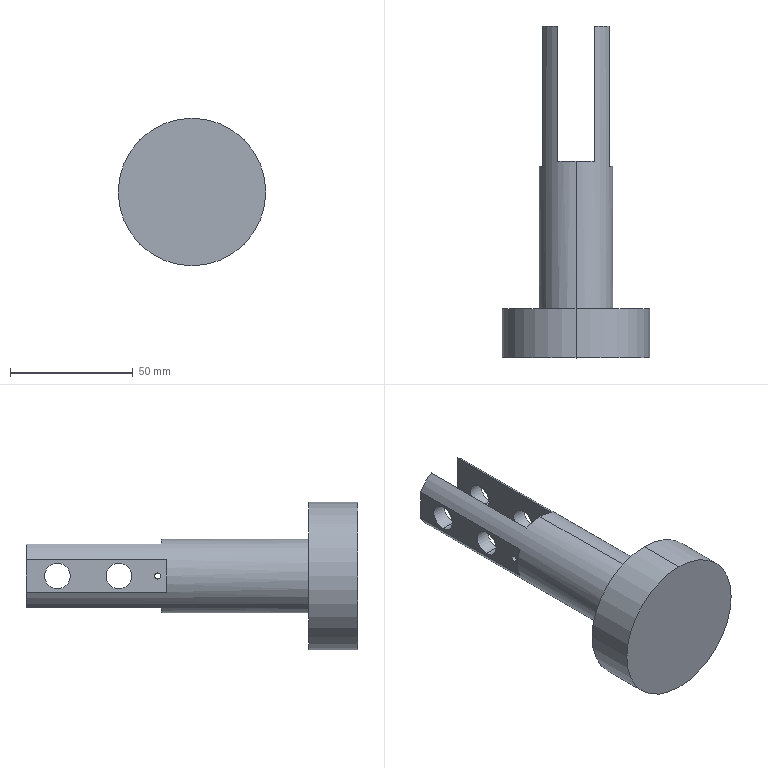Part | SolidWorks | features ICE 3, HoleWzd 2, Extrusion 1 | 1 solid | 27 faces | box 60 x 135 x 60 mm | volume 110518 mm3 | cylinder 16 | plane 11 | commonest cylinder face diameters 10.5 x8 2.5 x4 30 x2 60 x2
STEP:
#1=CARTESIAN_POINT('',(13.5,81.4,-1.25));
#2=VERTEX_POINT('',#1);
#3=CARTESIAN_POINT('',(13.5,81.4,1.25));
#4=VERTEX_POINT('',#3);
#5=CARTESIAN_POINT('',(13.5,81.4,0.));
#6=DIRECTION('',(-1.,0.,0.));
#7=DIRECTION('',(0.,0.,1.));
#8=AXIS2_PLACEMENT_3D('',#5,#6,#7);
#9=CIRCLE('',#8,1.25);
#10=EDGE_CURVE('',#2,#4,#9,.T.);
#11=ORIENTED_EDGE('',*,*,#10,.F.);
#12=CARTESIAN_POINT('',(7.5,81.4,-1.25));
#13=VERTEX_POINT('',#12);
#14=CARTESIAN_POINT('',(-13.5,81.4,-1.25));
#15=DIRECTION('',(-1.,0.,0.));
#16=VECTOR('',#15,1000.);
#17=LINE('',#14,#16);
#18=EDGE_CURVE('',#2,#13,#17,.T.);
#19=ORIENTED_EDGE('',*,*,#18,.T.);
#20=CARTESIAN_POINT('',(7.5,81.4,1.25));
#21=VERTEX_POINT('',#20);
#22=CARTESIAN_POINT('',(7.5,81.4,0.));
#23=DIRECTION('',(1.,0.,0.));
#24=DIRECTION('',(0.,0.,-1.));
#25=AXIS2_PLACEMENT_3D('',#22,#23,#24);
#26=CIRCLE('',#25,1.25);
#27=EDGE_CURVE('',#21,#13,#26,.T.);
#28=ORIENTED_EDGE('',*,*,#27,.F.);
#29=CARTESIAN_POINT('',(-13.5,81.4,1.25));
#30=DIRECTION('',(-1.,0.,0.));
#31=VECTOR('',#30,1000.);
#32=LINE('',#29,#31);
#33=EDGE_CURVE('',#4,#21,#32,.T.);
#34=ORIENTED_EDGE('',*,*,#33,.F.);
#35=EDGE_LOOP('',(#11,#19,#28,#34));
#36=FACE_OUTER_BOUND('',#35,.T.);
#37=CARTESIAN_POINT('',(-13.5,81.4,0.));
#38=DIRECTION('',(-1.,0.,0.));
#39=DIRECTION('',(0.,0.,1.));
#40=AXIS2_PLACEMENT_3D('',#37,#38,#39);
#41=CYLINDRICAL_SURFACE('',#40,1.25);
#42=ADVANCED_FACE('',(#36),#41,.F.);
#43=CARTESIAN_POINT('',(-7.5,81.4,-1.25));
#44=VERTEX_POINT('',#43);
#45=CARTESIAN_POINT('',(-7.5,81.4,1.25));
#46=VERTEX_POINT('',#45);
#47=CARTESIAN_POINT('',(-7.5,81.4,0.));
#48=DIRECTION('',(-1.,0.,0.));
#49=DIRECTION('',(0.,0.,1.));
#50=AXIS2_PLACEMENT_3D('',#47,#48,#49);
#51=CIRCLE('',#50,1.25);
#52=EDGE_CURVE('',#44,#46,#51,.T.);
#53=ORIENTED_EDGE('',*,*,#52,.F.);
#54=CARTESIAN_POINT('',(-13.5,81.4,-1.25));
#55=VERTEX_POINT('',#54);
#56=CARTESIAN_POINT('',(-13.5,81.4,-1.25));
#57=DIRECTION('',(-1.,0.,0.));
#58=VECTOR('',#57,1000.);
#59=LINE('',#56,#58);
#60=EDGE_CURVE('',#44,#55,#59,.T.);
#61=ORIENTED_EDGE('',*,*,#60,.T.);
#62=CARTESIAN_POINT('',(-13.5,81.4,1.25));
#63=VERTEX_POINT('',#62);
#64=CARTESIAN_POINT('',(-13.5,81.4,0.));
#65=DIRECTION('',(-1.,0.,0.));
#66=DIRECTION('',(0.,0.,1.));
#67=AXIS2_PLACEMENT_3D('',#64,#65,#66);
#68=CIRCLE('',#67,1.25);
#69=EDGE_CURVE('',#55,#63,#68,.T.);
#70=ORIENTED_EDGE('',*,*,#69,.T.);
#71=CARTESIAN_POINT('',(-13.5,81.4,1.25));
#72=DIRECTION('',(-1.,0.,0.));
#73=VECTOR('',#72,1000.);
#74=LINE('',#71,#73);
#75=EDGE_CURVE('',#46,#63,#74,.T.);
#76=ORIENTED_EDGE('',*,*,#75,.F.);
#77=EDGE_LOOP('',(#53,#61,#70,#76));
#78=FACE_OUTER_BOUND('',#77,.T.);
#79=CARTESIAN_POINT('',(-13.5,81.4,0.));
#80=DIRECTION('',(-1.,0.,0.));
#81=DIRECTION('',(0.,0.,1.));
#82=AXIS2_PLACEMENT_3D('',#79,#80,#81);
#83=CYLINDRICAL_SURFACE('',#82,1.25);
#84=ADVANCED_FACE('',(#78),#83,.F.);
#85=CARTESIAN_POINT('',(-13.5,97.25,5.25));
#86=VERTEX_POINT('',#85);
#87=CARTESIAN_POINT('',(-13.5,97.25,-5.25));
#88=VERTEX_POINT('',#87);
#89=CARTESIAN_POINT('',(-13.5,97.25,0.));
#90=DIRECTION('',(1.,0.,0.));
#91=DIRECTION('',(0.,1.,0.));
#92=AXIS2_PLACEMENT_3D('',#89,#90,#91);
#93=CIRCLE('',#92,5.25);
#94=EDGE_CURVE('',#86,#88,#93,.T.);
#95=ORIENTED_EDGE('',*,*,#94,.F.);
#96=CARTESIAN_POINT('',(-7.5,97.25,5.25));
#97=VERTEX_POINT('',#96);
#98=CARTESIAN_POINT('',(13.5,97.25,5.25));
#99=DIRECTION('',(1.,0.,0.));
#100=VECTOR('',#99,1000.);
#101=LINE('',#98,#100);
#102=EDGE_CURVE('',#86,#97,#101,.T.);
#103=ORIENTED_EDGE('',*,*,#102,.T.);
#104=CARTESIAN_POINT('',(-7.5,97.25,-5.25));
#105=VERTEX_POINT('',#104);
#106=CARTESIAN_POINT('',(-7.5,97.25,0.));
#107=DIRECTION('',(-1.,0.,0.));
#108=DIRECTION('',(0.,0.,1.));
#109=AXIS2_PLACEMENT_3D('',#106,#107,#108);
#110=CIRCLE('',#109,5.25);
#111=EDGE_CURVE('',#105,#97,#110,.T.);
#112=ORIENTED_EDGE('',*,*,#111,.F.);
#113=CARTESIAN_POINT('',(13.5,97.25,-5.25));
#114=DIRECTION('',(1.,0.,0.));
#115=VECTOR('',#114,1000.);
#116=LINE('',#113,#115);
#117=EDGE_CURVE('',#88,#105,#116,.T.);
#118=ORIENTED_EDGE('',*,*,#117,.F.);
#119=EDGE_LOOP('',(#95,#103,#112,#118));
#120=FACE_OUTER_BOUND('',#119,.T.);
#121=CARTESIAN_POINT('',(13.5,97.25,0.));
#122=DIRECTION('',(1.,0.,0.));
#123=DIRECTION('',(0.,0.,-1.));
#124=AXIS2_PLACEMENT_3D('',#121,#122,#123);
#125=CYLINDRICAL_SURFACE('',#124,5.25);
#126=ADVANCED_FACE('',(#120),#125,.F.);
#127=CARTESIAN_POINT('',(7.5,97.25,5.25));
#128=VERTEX_POINT('',#127);
#129=CARTESIAN_POINT('',(7.5,97.25,-5.25));
#130=VERTEX_POINT('',#129);
#131=CARTESIAN_POINT('',(7.5,97.25,0.));
#132=DIRECTION('',(1.,0.,0.));
#133=DIRECTION('',(0.,0.,-1.));
#134=AXIS2_PLACEMENT_3D('',#131,#132,#133);
#135=CIRCLE('',#134,5.25);
#136=EDGE_CURVE('',#128,#130,#135,.T.);
#137=ORIENTED_EDGE('',*,*,#136,.F.);
#138=CARTESIAN_POINT('',(13.5,97.25,5.25));
#139=VERTEX_POINT('',#138);
#140=CARTESIAN_POINT('',(13.5,97.25,5.25));
#141=DIRECTION('',(1.,0.,0.));
#142=VECTOR('',#141,1000.);
#143=LINE('',#140,#142);
#144=EDGE_CURVE('',#128,#139,#143,.T.);
#145=ORIENTED_EDGE('',*,*,#144,.T.);
#146=CARTESIAN_POINT('',(13.5,97.25,-5.25));
#147=VERTEX_POINT('',#146);
#148=CARTESIAN_POINT('',(13.5,97.25,0.));
#149=DIRECTION('',(1.,0.,0.));
#150=DIRECTION('',(0.,0.,-1.));
#151=AXIS2_PLACEMENT_3D('',#148,#149,#150);
#152=CIRCLE('',#151,5.25);
#153=EDGE_CURVE('',#139,#147,#152,.T.);
#154=ORIENTED_EDGE('',*,*,#153,.T.);
#155=CARTESIAN_POINT('',(13.5,97.25,-5.25));
#156=DIRECTION('',(1.,0.,0.));
#157=VECTOR('',#156,1000.);
#158=LINE('',#155,#157);
#159=EDGE_CURVE('',#130,#147,#158,.T.);
#160=ORIENTED_EDGE('',*,*,#159,.F.);
#161=EDGE_LOOP('',(#137,#145,#154,#160));
#162=FACE_OUTER_BOUND('',#161,.T.);
#163=CARTESIAN_POINT('',(13.5,97.25,0.));
#164=DIRECTION('',(1.,0.,0.));
#165=DIRECTION('',(0.,0.,-1.));
#166=AXIS2_PLACEMENT_3D('',#163,#164,#165);
#167=CYLINDRICAL_SURFACE('',#166,5.25);
#168=ADVANCED_FACE('',(#162),#167,.F.);
#169=CARTESIAN_POINT('',(7.5,122.25,5.25));
#170=VERTEX_POINT('',#169);
#171=CARTESIAN_POINT('',(7.5,122.25,-5.25));
#172=VERTEX_POINT('',#171);
#173=CARTESIAN_POINT('',(7.5,122.25,0.));
#174=DIRECTION('',(1.,0.,0.));
#175=DIRECTION('',(0.,0.,-1.));
#176=AXIS2_PLACEMENT_3D('',#173,#174,#175);
#177=CIRCLE('',#176,5.25);
#178=EDGE_CURVE('',#170,#172,#177,.T.);
#179=ORIENTED_EDGE('',*,*,#178,.F.);
#180=CARTESIAN_POINT('',(13.5,122.25,5.25));
#181=VERTEX_POINT('',#180);
#182=CARTESIAN_POINT('',(13.5,122.25,5.25));
#183=DIRECTION('',(1.,0.,0.));
#184=VECTOR('',#183,1000.);
#185=LINE('',#182,#184);
#186=EDGE_CURVE('',#170,#181,#185,.T.);
#187=ORIENTED_EDGE('',*,*,#186,.T.);
#188=CARTESIAN_POINT('',(13.5,122.25,-5.25));
#189=VERTEX_POINT('',#188);
#190=CARTESIAN_POINT('',(13.5,122.25,0.));
#191=DIRECTION('',(1.,0.,0.));
#192=DIRECTION('',(0.,0.,-1.));
#193=AXIS2_PLACEMENT_3D('',#190,#191,#192);
#194=CIRCLE('',#193,5.25);
#195=EDGE_CURVE('',#181,#189,#194,.T.);
#196=ORIENTED_EDGE('',*,*,#195,.T.);
#197=CARTESIAN_POINT('',(13.5,122.25,-5.25));
#198=DIRECTION('',(1.,0.,0.));
#199=VECTOR('',#198,1000.);
#200=LINE('',#197,#199);
#201=EDGE_CURVE('',#172,#189,#200,.T.);
#202=ORIENTED_EDGE('',*,*,#201,.F.);
#203=EDGE_LOOP('',(#179,#187,#196,#202));
#204=FACE_OUTER_BOUND('',#203,.T.);
#205=CARTESIAN_POINT('',(13.5,122.25,0.));
#206=DIRECTION('',(1.,0.,0.));
#207=DIRECTION('',(0.,0.,-1.));
#208=AXIS2_PLACEMENT_3D('',#205,#206,#207);
#209=CYLINDRICAL_SURFACE('',#208,5.25);
#210=ADVANCED_FACE('',(#204),#209,.F.);
#211=CARTESIAN_POINT('',(-13.5,122.25,5.25));
#212=VERTEX_POINT('',#211);
#213=CARTESIAN_POINT('',(-13.5,122.25,-5.25));
#214=VERTEX_POINT('',#213);
#215=CARTESIAN_POINT('',(-13.5,122.25,0.));
#216=DIRECTION('',(1.,0.,0.));
#217=DIRECTION('',(0.,1.,0.));
#218=AXIS2_PLACEMENT_3D('',#215,#216,#217);
#219=CIRCLE('',#218,5.25);
#220=EDGE_CURVE('',#212,#214,#219,.T.);
#221=ORIENTED_EDGE('',*,*,#220,.F.);
#222=CARTESIAN_POINT('',(-7.5,122.25,5.25));
#223=VERTEX_POINT('',#222);
#224=CARTESIAN_POINT('',(13.5,122.25,5.25));
#225=DIRECTION('',(1.,0.,0.));
#226=VECTOR('',#225,1000.);
#227=LINE('',#224,#226);
#228=EDGE_CURVE('',#212,#223,#227,.T.);
#229=ORIENTED_EDGE('',*,*,#228,.T.);
#230=CARTESIAN_POINT('',(-7.5,122.25,-5.25));
#231=VERTEX_POINT('',#230);
#232=CARTESIAN_POINT('',(-7.5,122.25,0.));
#233=DIRECTION('',(-1.,0.,0.));
#234=DIRECTION('',(0.,0.,1.));
#235=AXIS2_PLACEMENT_3D('',#232,#233,#234);
#236=CIRCLE('',#235,5.25);
#237=EDGE_CURVE('',#231,#223,#236,.T.);
#238=ORIENTED_EDGE('',*,*,#237,.F.);
#239=CARTESIAN_POINT('',(13.5,122.25,-5.25));
#240=DIRECTION('',(1.,0.,0.));
#241=VECTOR('',#240,1000.);
#242=LINE('',#239,#241);
#243=EDGE_CURVE('',#214,#231,#242,.T.);
#244=ORIENTED_EDGE('',*,*,#243,.F.);
#245=EDGE_LOOP('',(#221,#229,#238,#244));
#246=FACE_OUTER_BOUND('',#245,.T.);
#247=CARTESIAN_POINT('',(13.5,122.25,0.));
#248=DIRECTION('',(1.,0.,0.));
#249=DIRECTION('',(0.,0.,-1.));
#250=AXIS2_PLACEMENT_3D('',#247,#248,#249);
#251=CYLINDRICAL_SURFACE('',#250,5.25);
#252=ADVANCED_FACE('',(#246),#251,.F.);
#253=CARTESIAN_POINT('',(7.5,80.,12.99));
#254=VERTEX_POINT('',#253);
#255=CARTESIAN_POINT('',(0.,80.,15.));
#256=VERTEX_POINT('',#255);
#257=CARTESIAN_POINT('',(0.,80.,0.));
#258=DIRECTION('',(0.,-1.,0.));
#259=DIRECTION('',(0.,0.,-1.));
#260=AXIS2_PLACEMENT_3D('',#257,#258,#259);
#261=CIRCLE('',#260,15.);
#262=EDGE_CURVE('',#254,#256,#261,.T.);
#263=ORIENTED_EDGE('',*,*,#262,.T.);
#264=CARTESIAN_POINT('',(0.,20.,15.));
#265=VERTEX_POINT('',#264);
#266=CARTESIAN_POINT('',(0.,135.,15.));
#267=DIRECTION('',(0.,-1.,0.));
#268=VECTOR('',#267,1000.);
#269=LINE('',#266,#268);
#270=EDGE_CURVE('',#256,#265,#269,.T.);
#271=ORIENTED_EDGE('',*,*,#270,.T.);
#272=CARTESIAN_POINT('',(0.,20.,-15.));
#273=VERTEX_POINT('',#272);
#274=CARTESIAN_POINT('',(0.,20.,0.));
#275=DIRECTION('',(0.,1.,0.));
#276=DIRECTION('',(0.,0.,1.));
#277=AXIS2_PLACEMENT_3D('',#274,#275,#276);
#278=CIRCLE('',#277,15.);
#279=EDGE_CURVE('',#265,#273,#278,.T.);
#280=ORIENTED_EDGE('',*,*,#279,.T.);
#281=CARTESIAN_POINT('',(0.,80.,-15.));
#282=VERTEX_POINT('',#281);
#283=CARTESIAN_POINT('',(0.,135.,-15.));
#284=DIRECTION('',(0.,-1.,0.));
#285=VECTOR('',#284,1000.);
#286=LINE('',#283,#285);
#287=EDGE_CURVE('',#282,#273,#286,.T.);
#288=ORIENTED_EDGE('',*,*,#287,.F.);
#289=CARTESIAN_POINT('',(7.5,80.,-12.99));
#290=VERTEX_POINT('',#289);
#291=CARTESIAN_POINT('',(0.,80.,0.));
#292=DIRECTION('',(0.,-1.,0.));
#293=DIRECTION('',(0.,0.,-1.));
#294=AXIS2_PLACEMENT_3D('',#291,#292,#293);
#295=CIRCLE('',#294,15.);
#296=EDGE_CURVE('',#282,#290,#295,.T.);
#297=ORIENTED_EDGE('',*,*,#296,.T.);
#298=CARTESIAN_POINT('',(7.5,135.,-12.99));
#299=VERTEX_POINT('',#298);
#300=CARTESIAN_POINT('',(7.5,135.,-12.99));
#301=DIRECTION('',(0.,1.,0.));
#302=VECTOR('',#301,1000.);
#303=LINE('',#300,#302);
#304=EDGE_CURVE('',#290,#299,#303,.T.);
#305=ORIENTED_EDGE('',*,*,#304,.T.);
#306=CARTESIAN_POINT('',(13.5,135.,-6.538));
#307=VERTEX_POINT('',#306);
#308=CARTESIAN_POINT('',(0.,135.,0.));
#309=DIRECTION('',(0.,1.,0.));
#310=DIRECTION('',(0.,0.,1.));
#311=AXIS2_PLACEMENT_3D('',#308,#309,#310);
#312=CIRCLE('',#311,15.);
#313=EDGE_CURVE('',#307,#299,#312,.T.);
#314=ORIENTED_EDGE('',*,*,#313,.F.);
#315=CARTESIAN_POINT('',(13.5,78.,-6.538));
#316=VERTEX_POINT('',#315);
#317=CARTESIAN_POINT('',(13.5,135.,-6.538));
#318=DIRECTION('',(0.,-1.,0.));
#319=VECTOR('',#318,1000.);
#320=LINE('',#317,#319);
#321=EDGE_CURVE('',#307,#316,#320,.T.);
#322=ORIENTED_EDGE('',*,*,#321,.T.);
#323=CARTESIAN_POINT('',(13.5,78.,6.538));
#324=VERTEX_POINT('',#323);
#325=CARTESIAN_POINT('',(0.,78.,0.));
#326=DIRECTION('',(0.,-1.,0.));
#327=DIRECTION('',(0.,0.,-1.));
#328=AXIS2_PLACEMENT_3D('',#325,#326,#327);
#329=CIRCLE('',#328,15.);
#330=EDGE_CURVE('',#316,#324,#329,.T.);
#331=ORIENTED_EDGE('',*,*,#330,.T.);
#332=CARTESIAN_POINT('',(13.5,135.,6.538));
#333=VERTEX_POINT('',#332);
#334=CARTESIAN_POINT('',(13.5,135.,6.538));
#335=DIRECTION('',(0.,1.,0.));
#336=VECTOR('',#335,1000.);
#337=LINE('',#334,#336);
#338=EDGE_CURVE('',#324,#333,#337,.T.);
#339=ORIENTED_EDGE('',*,*,#338,.T.);
#340=CARTESIAN_POINT('',(7.5,135.,12.99));
#341=VERTEX_POINT('',#340);
#342=CARTESIAN_POINT('',(0.,135.,0.));
#343=DIRECTION('',(0.,1.,0.));
#344=DIRECTION('',(0.,0.,1.));
#345=AXIS2_PLACEMENT_3D('',#342,#343,#344);
#346=CIRCLE('',#345,15.);
#347=EDGE_CURVE('',#341,#333,#346,.T.);
#348=ORIENTED_EDGE('',*,*,#347,.F.);
#349=CARTESIAN_POINT('',(7.5,135.,12.99));
#350=DIRECTION('',(0.,-1.,0.));
#351=VECTOR('',#350,1000.);
#352=LINE('',#349,#351);
#353=EDGE_CURVE('',#341,#254,#352,.T.);
#354=ORIENTED_EDGE('',*,*,#353,.T.);
#355=EDGE_LOOP('',(#263,#271,#280,#288,#297,#305,#314,#322,#331,#339,#348,#354));
#356=FACE_OUTER_BOUND('',#355,.T.);
#357=CARTESIAN_POINT('',(0.,135.,0.));
#358=DIRECTION('',(0.,-1.,0.));
#359=DIRECTION('',(0.,0.,-1.));
#360=AXIS2_PLACEMENT_3D('',#357,#358,#359);
#361=CYLINDRICAL_SURFACE('',#360,15.);
#362=ADVANCED_FACE('',(#356),#361,.T.);
#363=CARTESIAN_POINT('',(0.,20.,30.));
#364=VERTEX_POINT('',#363);
#365=CARTESIAN_POINT('',(0.,20.,-30.));
#366=VERTEX_POINT('',#365);
#367=CARTESIAN_POINT('',(0.,20.,0.));
#368=DIRECTION('',(0.,1.,0.));
#369=DIRECTION('',(0.,0.,1.));
#370=AXIS2_PLACEMENT_3D('',#367,#368,#369);
#371=CIRCLE('',#370,30.);
#372=EDGE_CURVE('',#364,#366,#371,.T.);
#373=ORIENTED_EDGE('',*,*,#372,.F.);
#374=CARTESIAN_POINT('',(0.,0.,30.));
#375=VERTEX_POINT('',#374);
#376=CARTESIAN_POINT('',(0.,20.,30.));
#377=DIRECTION('',(0.,-1.,0.));
#378=VECTOR('',#377,1000.);
#379=LINE('',#376,#378);
#380=EDGE_CURVE('',#364,#375,#379,.T.);
#381=ORIENTED_EDGE('',*,*,#380,.T.);
#382=CARTESIAN_POINT('',(0.,0.,-30.));
#383=VERTEX_POINT('',#382);
#384=CARTESIAN_POINT('',(0.,0.,0.));
#385=DIRECTION('',(0.,1.,0.));
#386=DIRECTION('',(0.,0.,1.));
#387=AXIS2_PLACEMENT_3D('',#384,#385,#386);
#388=CIRCLE('',#387,30.);
#389=EDGE_CURVE('',#375,#383,#388,.T.);
#390=ORIENTED_EDGE('',*,*,#389,.T.);
#391=CARTESIAN_POINT('',(0.,20.,-30.));
#392=DIRECTION('',(0.,-1.,0.));
#393=VECTOR('',#392,1000.);
#394=LINE('',#391,#393);
#395=EDGE_CURVE('',#366,#383,#394,.T.);
#396=ORIENTED_EDGE('',*,*,#395,.F.);
#397=EDGE_LOOP('',(#373,#381,#390,#396));
#398=FACE_OUTER_BOUND('',#397,.T.);
#399=CARTESIAN_POINT('',(0.,20.,0.));
#400=DIRECTION('',(0.,-1.,0.));
#401=DIRECTION('',(0.,0.,-1.));
#402=AXIS2_PLACEMENT_3D('',#399,#400,#401);
#403=CYLINDRICAL_SURFACE('',#402,30.);
#404=ADVANCED_FACE('',(#398),#403,.T.);
#405=CARTESIAN_POINT('',(-13.5,135.,6.538));
#406=VERTEX_POINT('',#405);
#407=CARTESIAN_POINT('',(-13.5,135.,-6.538));
#408=VERTEX_POINT('',#407);
#409=CARTESIAN_POINT('',(-13.5,135.,0.));
#410=DIRECTION('',(0.,0.,-1.));
#411=VECTOR('',#410,1000.);
#412=LINE('',#409,#411);
#413=EDGE_CURVE('',#406,#408,#412,.T.);
#414=ORIENTED_EDGE('',*,*,#413,.F.);
#415=CARTESIAN_POINT('',(-7.5,135.,12.99));
#416=VERTEX_POINT('',#415);
#417=CARTESIAN_POINT('',(0.,135.,0.));
#418=DIRECTION('',(0.,1.,0.));
#419=DIRECTION('',(0.,0.,1.));
#420=AXIS2_PLACEMENT_3D('',#417,#418,#419);
#421=CIRCLE('',#420,15.);
#422=EDGE_CURVE('',#406,#416,#421,.T.);
#423=ORIENTED_EDGE('',*,*,#422,.T.);
#424=CARTESIAN_POINT('',(-7.5,135.,-12.99));
#425=VERTEX_POINT('',#424);
#426=CARTESIAN_POINT('',(-7.5,135.,0.));
#427=DIRECTION('',(0.,0.,1.));
#428=VECTOR('',#427,1000.);
#429=LINE('',#426,#428);
#430=EDGE_CURVE('',#425,#416,#429,.T.);
#431=ORIENTED_EDGE('',*,*,#430,.F.);
#432=CARTESIAN_POINT('',(0.,135.,0.));
#433=DIRECTION('',(0.,1.,0.));
#434=DIRECTION('',(0.,0.,1.));
#435=AXIS2_PLACEMENT_3D('',#432,#433,#434);
#436=CIRCLE('',#435,15.);
#437=EDGE_CURVE('',#425,#408,#436,.T.);
#438=ORIENTED_EDGE('',*,*,#437,.T.);
#439=EDGE_LOOP('',(#414,#423,#431,#438));
#440=FACE_OUTER_BOUND('',#439,.T.);
#441=CARTESIAN_POINT('',(0.,135.,0.));
#442=DIRECTION('',(0.,1.,0.));
#443=DIRECTION('',(0.,0.,1.));
#444=AXIS2_PLACEMENT_3D('',#441,#442,#443);
#445=PLANE('',#444);
#446=ADVANCED_FACE('',(#440),#445,.T.);
#447=ORIENTED_EDGE('',*,*,#380,.F.);
#448=CARTESIAN_POINT('',(0.,20.,0.));
#449=DIRECTION('',(0.,1.,0.));
#450=DIRECTION('',(0.,0.,1.));
#451=AXIS2_PLACEMENT_3D('',#448,#449,#450);
#452=CIRCLE('',#451,30.);
#453=EDGE_CURVE('',#366,#364,#452,.T.);
#454=ORIENTED_EDGE('',*,*,#453,.F.);
#455=ORIENTED_EDGE('',*,*,#395,.T.);
#456=CARTESIAN_POINT('',(0.,0.,0.));
#457=DIRECTION('',(0.,1.,0.));
#458=DIRECTION('',(0.,0.,1.));
#459=AXIS2_PLACEMENT_3D('',#456,#457,#458);
#460=CIRCLE('',#459,30.);
#461=EDGE_CURVE('',#383,#375,#460,.T.);
#462=ORIENTED_EDGE('',*,*,#461,.T.);
#463=EDGE_LOOP('',(#447,#454,#455,#462));
#464=FACE_OUTER_BOUND('',#463,.T.);
#465=CARTESIAN_POINT('',(0.,20.,0.));
#466=DIRECTION('',(0.,-1.,0.));
#467=DIRECTION('',(0.,0.,-1.));
#468=AXIS2_PLACEMENT_3D('',#465,#466,#467);
#469=CYLINDRICAL_SURFACE('',#468,30.);
#470=ADVANCED_FACE('',(#464),#469,.T.);
#471=CARTESIAN_POINT('',(0.,20.,0.));
#472=DIRECTION('',(0.,1.,0.));
#473=DIRECTION('',(0.,0.,1.));
#474=AXIS2_PLACEMENT_3D('',#471,#472,#473);
#475=CIRCLE('',#474,15.);
#476=EDGE_CURVE('',#273,#265,#475,.T.);
#477=ORIENTED_EDGE('',*,*,#476,.F.);
#478=ORIENTED_EDGE('',*,*,#279,.F.);
#479=EDGE_LOOP('',(#477,#478));
#480=FACE_BOUND('',#479,.T.);
#481=ORIENTED_EDGE('',*,*,#453,.T.);
#482=ORIENTED_EDGE('',*,*,#372,.T.);
#483=EDGE_LOOP('',(#481,#482));
#484=FACE_OUTER_BOUND('',#483,.T.);
#485=CARTESIAN_POINT('',(0.,20.,0.));
#486=DIRECTION('',(0.,1.,0.));
#487=DIRECTION('',(0.,0.,1.));
#488=AXIS2_PLACEMENT_3D('',#485,#486,#487);
#489=PLANE('',#488);
#490=ADVANCED_FACE('',(#480,#484),#489,.T.);
#491=ORIENTED_EDGE('',*,*,#461,.F.);
#492=ORIENTED_EDGE('',*,*,#389,.F.);
#493=EDGE_LOOP('',(#491,#492));
#494=FACE_OUTER_BOUND('',#493,.T.);
#495=CARTESIAN_POINT('',(0.,0.,0.));
#496=DIRECTION('',(0.,1.,0.));
#497=DIRECTION('',(0.,0.,1.));
#498=AXIS2_PLACEMENT_3D('',#495,#496,#497);
#499=PLANE('',#498);
#500=ADVANCED_FACE('',(#494),#499,.F.);
#501=ORIENTED_EDGE('',*,*,#270,.F.);
#502=CARTESIAN_POINT('',(-7.5,80.,12.99));
#503=VERTEX_POINT('',#502);
#504=CARTESIAN_POINT('',(0.,80.,0.));
#505=DIRECTION('',(0.,-1.,0.));
#506=DIRECTION('',(0.,0.,-1.));
#507=AXIS2_PLACEMENT_3D('',#504,#505,#506);
#508=CIRCLE('',#507,15.);
#509=EDGE_CURVE('',#256,#503,#508,.T.);
#510=ORIENTED_EDGE('',*,*,#509,.T.);
#511=CARTESIAN_POINT('',(-7.5,135.,12.99));
#512=DIRECTION('',(0.,1.,0.));
#513=VECTOR('',#512,1000.);
#514=LINE('',#511,#513);
#515=EDGE_CURVE('',#503,#416,#514,.T.);
#516=ORIENTED_EDGE('',*,*,#515,.T.);
#517=ORIENTED_EDGE('',*,*,#422,.F.);
#518=CARTESIAN_POINT('',(-13.5,78.,6.538));
#519=VERTEX_POINT('',#518);
#520=CARTESIAN_POINT('',(-13.5,135.,6.538));
#521=DIRECTION('',(0.,-1.,0.));
#522=VECTOR('',#521,1000.);
#523=LINE('',#520,#522);
#524=EDGE_CURVE('',#406,#519,#523,.T.);
#525=ORIENTED_EDGE('',*,*,#524,.T.);
#526=CARTESIAN_POINT('',(-13.5,78.,-6.538));
#527=VERTEX_POINT('',#526);
#528=CARTESIAN_POINT('',(0.,78.,0.));
#529=DIRECTION('',(0.,-1.,0.));
#530=DIRECTION('',(0.,0.,-1.));
#531=AXIS2_PLACEMENT_3D('',#528,#529,#530);
#532=CIRCLE('',#531,15.);
#533=EDGE_CURVE('',#519,#527,#532,.T.);
#534=ORIENTED_EDGE('',*,*,#533,.T.);
#535=CARTESIAN_POINT('',(-13.5,135.,-6.538));
#536=DIRECTION('',(0.,1.,0.));
#537=VECTOR('',#536,1000.);
#538=LINE('',#535,#537);
#539=EDGE_CURVE('',#527,#408,#538,.T.);
#540=ORIENTED_EDGE('',*,*,#539,.T.);
#541=ORIENTED_EDGE('',*,*,#437,.F.);
#542=CARTESIAN_POINT('',(-7.5,80.,-12.99));
#543=VERTEX_POINT('',#542);
#544=CARTESIAN_POINT('',(-7.5,135.,-12.99));
#545=DIRECTION('',(0.,-1.,0.));
#546=VECTOR('',#545,1000.);
#547=LINE('',#544,#546);
#548=EDGE_CURVE('',#425,#543,#547,.T.);
#549=ORIENTED_EDGE('',*,*,#548,.T.);
#550=CARTESIAN_POINT('',(0.,80.,0.));
#551=DIRECTION('',(0.,-1.,0.));
#552=DIRECTION('',(0.,0.,-1.));
#553=AXIS2_PLACEMENT_3D('',#550,#551,#552);
#554=CIRCLE('',#553,15.);
#555=EDGE_CURVE('',#543,#282,#554,.T.);
#556=ORIENTED_EDGE('',*,*,#555,.T.);
#557=ORIENTED_EDGE('',*,*,#287,.T.);
#558=ORIENTED_EDGE('',*,*,#476,.T.);
#559=EDGE_LOOP('',(#501,#510,#516,#517,#525,#534,#540,#541,#549,#556,#557,#558));
#560=FACE_OUTER_BOUND('',#559,.T.);
#561=CARTESIAN_POINT('',(0.,135.,0.));
#562=DIRECTION('',(0.,-1.,0.));
#563=DIRECTION('',(0.,0.,-1.));
#564=AXIS2_PLACEMENT_3D('',#561,#562,#563);
#565=CYLINDRICAL_SURFACE('',#564,15.);
#566=ADVANCED_FACE('',(#560),#565,.T.);
#567=CARTESIAN_POINT('',(13.5,135.,0.));
#568=DIRECTION('',(0.,0.,1.));
#569=VECTOR('',#568,1000.);
#570=LINE('',#567,#569);
#571=EDGE_CURVE('',#307,#333,#570,.T.);
#572=ORIENTED_EDGE('',*,*,#571,.F.);
#573=ORIENTED_EDGE('',*,*,#313,.T.);
#574=CARTESIAN_POINT('',(7.5,135.,0.));
#575=DIRECTION('',(0.,0.,-1.));
#576=VECTOR('',#575,1000.);
#577=LINE('',#574,#576);
#578=EDGE_CURVE('',#341,#299,#577,.T.);
#579=ORIENTED_EDGE('',*,*,#578,.F.);
#580=ORIENTED_EDGE('',*,*,#347,.T.);
#581=EDGE_LOOP('',(#572,#573,#579,#580));
#582=FACE_OUTER_BOUND('',#581,.T.);
#583=CARTESIAN_POINT('',(0.,135.,0.));
#584=DIRECTION('',(0.,1.,0.));
#585=DIRECTION('',(0.,0.,1.));
#586=AXIS2_PLACEMENT_3D('',#583,#584,#585);
#587=PLANE('',#586);
#588=ADVANCED_FACE('',(#582),#587,.T.);
#589=CARTESIAN_POINT('',(7.5,80.,-50.));
#590=DIRECTION('',(0.,0.,1.));
#591=VECTOR('',#590,1000.);
#592=LINE('',#589,#591);
#593=EDGE_CURVE('',#290,#254,#592,.T.);
#594=ORIENTED_EDGE('',*,*,#593,.F.);
#595=ORIENTED_EDGE('',*,*,#296,.F.);
#596=ORIENTED_EDGE('',*,*,#555,.F.);
#597=CARTESIAN_POINT('',(-7.5,80.,-50.));
#598=DIRECTION('',(0.,0.,1.));
#599=VECTOR('',#598,1000.);
#600=LINE('',#597,#599);
#601=EDGE_CURVE('',#543,#503,#600,.T.);
#602=ORIENTED_EDGE('',*,*,#601,.T.);
#603=ORIENTED_EDGE('',*,*,#509,.F.);
#604=ORIENTED_EDGE('',*,*,#262,.F.);
#605=EDGE_LOOP('',(#594,#595,#596,#602,#603,#604));
#606=FACE_OUTER_BOUND('',#605,.T.);
#607=CARTESIAN_POINT('',(-7.5,80.,-50.));
#608=DIRECTION('',(0.,-1.,0.));
#609=DIRECTION('',(0.,0.,-1.));
#610=AXIS2_PLACEMENT_3D('',#607,#608,#609);
#611=PLANE('',#610);
#612=ADVANCED_FACE('',(#606),#611,.F.);
#613=CARTESIAN_POINT('',(-7.5,81.4,0.));
#614=DIRECTION('',(-1.,0.,0.));
#615=DIRECTION('',(0.,0.,1.));
#616=AXIS2_PLACEMENT_3D('',#613,#614,#615);
#617=CIRCLE('',#616,1.25);
#618=EDGE_CURVE('',#46,#44,#617,.T.);
#619=ORIENTED_EDGE('',*,*,#618,.T.);
#620=ORIENTED_EDGE('',*,*,#52,.T.);
#621=EDGE_LOOP('',(#619,#620));
#622=FACE_BOUND('',#621,.T.);
#623=ORIENTED_EDGE('',*,*,#111,.T.);
#624=CARTESIAN_POINT('',(-7.5,97.25,0.));
#625=DIRECTION('',(-1.,0.,0.));
#626=DIRECTION('',(0.,0.,1.));
#627=AXIS2_PLACEMENT_3D('',#624,#625,#626);
#628=CIRCLE('',#627,5.25);
#629=EDGE_CURVE('',#97,#105,#628,.T.);
#630=ORIENTED_EDGE('',*,*,#629,.T.);
#631=EDGE_LOOP('',(#623,#630));
#632=FACE_BOUND('',#631,.T.);
#633=ORIENTED_EDGE('',*,*,#237,.T.);
#634=CARTESIAN_POINT('',(-7.5,122.25,0.));
#635=DIRECTION('',(-1.,0.,0.));
#636=DIRECTION('',(0.,0.,1.));
#637=AXIS2_PLACEMENT_3D('',#634,#635,#636);
#638=CIRCLE('',#637,5.25);
#639=EDGE_CURVE('',#223,#231,#638,.T.);
#640=ORIENTED_EDGE('',*,*,#639,.T.);
#641=EDGE_LOOP('',(#633,#640));
#642=FACE_BOUND('',#641,.T.);
#643=ORIENTED_EDGE('',*,*,#430,.T.);
#644=ORIENTED_EDGE('',*,*,#515,.F.);
#645=ORIENTED_EDGE('',*,*,#601,.F.);
#646=ORIENTED_EDGE('',*,*,#548,.F.);
#647=EDGE_LOOP('',(#643,#644,#645,#646));
#648=FACE_OUTER_BOUND('',#647,.T.);
#649=CARTESIAN_POINT('',(-7.5,80.,-50.));
#650=DIRECTION('',(-1.,0.,0.));
#651=DIRECTION('',(0.,0.,1.));
#652=AXIS2_PLACEMENT_3D('',#649,#650,#651);
#653=PLANE('',#652);
#654=ADVANCED_FACE('',(#622,#632,#642,#648),#653,.F.);
#655=ORIENTED_EDGE('',*,*,#27,.T.);
#656=CARTESIAN_POINT('',(7.5,81.4,0.));
#657=DIRECTION('',(1.,0.,0.));
#658=DIRECTION('',(0.,0.,-1.));
#659=AXIS2_PLACEMENT_3D('',#656,#657,#658);
#660=CIRCLE('',#659,1.25);
#661=EDGE_CURVE('',#13,#21,#660,.T.);
#662=ORIENTED_EDGE('',*,*,#661,.T.);
#663=EDGE_LOOP('',(#655,#662));
#664=FACE_BOUND('',#663,.T.);
#665=CARTESIAN_POINT('',(7.5,97.25,0.));
#666=DIRECTION('',(1.,0.,0.));
#667=DIRECTION('',(0.,0.,-1.));
#668=AXIS2_PLACEMENT_3D('',#665,#666,#667);
#669=CIRCLE('',#668,5.25);
#670=EDGE_CURVE('',#130,#128,#669,.T.);
#671=ORIENTED_EDGE('',*,*,#670,.T.);
#672=ORIENTED_EDGE('',*,*,#136,.T.);
#673=EDGE_LOOP('',(#671,#672));
#674=FACE_BOUND('',#673,.T.);
#675=CARTESIAN_POINT('',(7.5,122.25,0.));
#676=DIRECTION('',(1.,0.,0.));
#677=DIRECTION('',(0.,0.,-1.));
#678=AXIS2_PLACEMENT_3D('',#675,#676,#677);
#679=CIRCLE('',#678,5.25);
#680=EDGE_CURVE('',#172,#170,#679,.T.);
#681=ORIENTED_EDGE('',*,*,#680,.T.);
#682=ORIENTED_EDGE('',*,*,#178,.T.);
#683=EDGE_LOOP('',(#681,#682));
#684=FACE_BOUND('',#683,.T.);
#685=ORIENTED_EDGE('',*,*,#578,.T.);
#686=ORIENTED_EDGE('',*,*,#304,.F.);
#687=ORIENTED_EDGE('',*,*,#593,.T.);
#688=ORIENTED_EDGE('',*,*,#353,.F.);
#689=EDGE_LOOP('',(#685,#686,#687,#688));
#690=FACE_OUTER_BOUND('',#689,.T.);
#691=CARTESIAN_POINT('',(7.5,80.,-50.));
#692=DIRECTION('',(1.,0.,0.));
#693=DIRECTION('',(0.,0.,-1.));
#694=AXIS2_PLACEMENT_3D('',#691,#692,#693);
#695=PLANE('',#694);
#696=ADVANCED_FACE('',(#664,#674,#684,#690),#695,.F.);
#697=CARTESIAN_POINT('',(13.5,78.,-25.));
#698=DIRECTION('',(0.,0.,1.));
#699=VECTOR('',#698,1000.);
#700=LINE('',#697,#699);
#701=EDGE_CURVE('',#316,#324,#700,.T.);
#702=ORIENTED_EDGE('',*,*,#701,.T.);
#703=ORIENTED_EDGE('',*,*,#330,.F.);
#704=EDGE_LOOP('',(#702,#703));
#705=FACE_OUTER_BOUND('',#704,.T.);
#706=CARTESIAN_POINT('',(24.715,78.,-25.));
#707=DIRECTION('',(0.,-1.,0.));
#708=DIRECTION('',(0.,0.,-1.));
#709=AXIS2_PLACEMENT_3D('',#706,#707,#708);
#710=PLANE('',#709);
#711=ADVANCED_FACE('',(#705),#710,.F.);
#712=CARTESIAN_POINT('',(13.5,81.4,0.));
#713=DIRECTION('',(-1.,0.,0.));
#714=DIRECTION('',(0.,0.,1.));
#715=AXIS2_PLACEMENT_3D('',#712,#713,#714);
#716=CIRCLE('',#715,1.25);
#717=EDGE_CURVE('',#4,#2,#716,.T.);
#718=ORIENTED_EDGE('',*,*,#717,.T.);
#719=ORIENTED_EDGE('',*,*,#10,.T.);
#720=EDGE_LOOP('',(#718,#719));
#721=FACE_BOUND('',#720,.T.);
#722=CARTESIAN_POINT('',(13.5,97.25,0.));
#723=DIRECTION('',(1.,0.,0.));
#724=DIRECTION('',(0.,0.,-1.));
#725=AXIS2_PLACEMENT_3D('',#722,#723,#724);
#726=CIRCLE('',#725,5.25);
#727=EDGE_CURVE('',#147,#139,#726,.T.);
#728=ORIENTED_EDGE('',*,*,#727,.F.);
#729=ORIENTED_EDGE('',*,*,#153,.F.);
#730=EDGE_LOOP('',(#728,#729));
#731=FACE_BOUND('',#730,.T.);
#732=CARTESIAN_POINT('',(13.5,122.25,0.));
#733=DIRECTION('',(1.,0.,0.));
#734=DIRECTION('',(0.,0.,-1.));
#735=AXIS2_PLACEMENT_3D('',#732,#733,#734);
#736=CIRCLE('',#735,5.25);
#737=EDGE_CURVE('',#189,#181,#736,.T.);
#738=ORIENTED_EDGE('',*,*,#737,.F.);
#739=ORIENTED_EDGE('',*,*,#195,.F.);
#740=EDGE_LOOP('',(#738,#739));
#741=FACE_BOUND('',#740,.T.);
#742=ORIENTED_EDGE('',*,*,#571,.T.);
#743=ORIENTED_EDGE('',*,*,#338,.F.);
#744=ORIENTED_EDGE('',*,*,#701,.F.);
#745=ORIENTED_EDGE('',*,*,#321,.F.);
#746=EDGE_LOOP('',(#742,#743,#744,#745));
#747=FACE_OUTER_BOUND('',#746,.T.);
#748=CARTESIAN_POINT('',(13.5,78.,-25.));
#749=DIRECTION('',(-1.,0.,0.));
#750=DIRECTION('',(0.,0.,1.));
#751=AXIS2_PLACEMENT_3D('',#748,#749,#750);
#752=PLANE('',#751);
#753=ADVANCED_FACE('',(#721,#731,#741,#747),#752,.F.);
#754=CARTESIAN_POINT('',(-13.5,81.4,0.));
#755=DIRECTION('',(-1.,0.,0.));
#756=DIRECTION('',(0.,0.,1.));
#757=AXIS2_PLACEMENT_3D('',#754,#755,#756);
#758=CIRCLE('',#757,1.25);
#759=EDGE_CURVE('',#63,#55,#758,.T.);
#760=ORIENTED_EDGE('',*,*,#759,.F.);
#761=ORIENTED_EDGE('',*,*,#69,.F.);
#762=EDGE_LOOP('',(#760,#761));
#763=FACE_BOUND('',#762,.T.);
#764=CARTESIAN_POINT('',(-13.5,97.25,0.));
#765=DIRECTION('',(1.,0.,0.));
#766=DIRECTION('',(0.,1.,0.));
#767=AXIS2_PLACEMENT_3D('',#764,#765,#766);
#768=CIRCLE('',#767,5.25);
#769=EDGE_CURVE('',#88,#86,#768,.T.);
#770=ORIENTED_EDGE('',*,*,#769,.T.);
#771=ORIENTED_EDGE('',*,*,#94,.T.);
#772=EDGE_LOOP('',(#770,#771));
#773=FACE_BOUND('',#772,.T.);
#774=CARTESIAN_POINT('',(-13.5,122.25,0.));
#775=DIRECTION('',(1.,0.,0.));
#776=DIRECTION('',(0.,1.,0.));
#777=AXIS2_PLACEMENT_3D('',#774,#775,#776);
#778=CIRCLE('',#777,5.25);
#779=EDGE_CURVE('',#214,#212,#778,.T.);
#780=ORIENTED_EDGE('',*,*,#779,.T.);
#781=ORIENTED_EDGE('',*,*,#220,.T.);
#782=EDGE_LOOP('',(#780,#781));
#783=FACE_BOUND('',#782,.T.);
#784=ORIENTED_EDGE('',*,*,#413,.T.);
#785=ORIENTED_EDGE('',*,*,#539,.F.);
#786=CARTESIAN_POINT('',(-13.5,78.,-25.));
#787=DIRECTION('',(0.,0.,1.));
#788=VECTOR('',#787,1000.);
#789=LINE('',#786,#788);
#790=EDGE_CURVE('',#527,#519,#789,.T.);
#791=ORIENTED_EDGE('',*,*,#790,.T.);
#792=ORIENTED_EDGE('',*,*,#524,.F.);
#793=EDGE_LOOP('',(#784,#785,#791,#792));
#794=FACE_OUTER_BOUND('',#793,.T.);
#795=CARTESIAN_POINT('',(-13.5,78.,-25.));
#796=DIRECTION('',(1.,0.,0.));
#797=DIRECTION('',(0.,1.,0.));
#798=AXIS2_PLACEMENT_3D('',#795,#796,#797);
#799=PLANE('',#798);
#800=ADVANCED_FACE('',(#763,#773,#783,#794),#799,.F.);
#801=ORIENTED_EDGE('',*,*,#790,.F.);
#802=ORIENTED_EDGE('',*,*,#533,.F.);
#803=EDGE_LOOP('',(#801,#802));
#804=FACE_OUTER_BOUND('',#803,.T.);
#805=CARTESIAN_POINT('',(-24.715,78.,-25.));
#806=DIRECTION('',(0.,-1.,0.));
#807=DIRECTION('',(0.,0.,-1.));
#808=AXIS2_PLACEMENT_3D('',#805,#806,#807);
#809=PLANE('',#808);
#810=ADVANCED_FACE('',(#804),#809,.F.);
#811=ORIENTED_EDGE('',*,*,#228,.F.);
#812=ORIENTED_EDGE('',*,*,#779,.F.);
#813=ORIENTED_EDGE('',*,*,#243,.T.);
#814=ORIENTED_EDGE('',*,*,#639,.F.);
#815=EDGE_LOOP('',(#811,#812,#813,#814));
#816=FACE_OUTER_BOUND('',#815,.T.);
#817=CARTESIAN_POINT('',(13.5,122.25,0.));
#818=DIRECTION('',(1.,0.,0.));
#819=DIRECTION('',(0.,0.,-1.));
#820=AXIS2_PLACEMENT_3D('',#817,#818,#819);
#821=CYLINDRICAL_SURFACE('',#820,5.25);
#822=ADVANCED_FACE('',(#816),#821,.F.);
#823=ORIENTED_EDGE('',*,*,#186,.F.);
#824=ORIENTED_EDGE('',*,*,#680,.F.);
#825=ORIENTED_EDGE('',*,*,#201,.T.);
#826=ORIENTED_EDGE('',*,*,#737,.T.);
#827=EDGE_LOOP('',(#823,#824,#825,#826));
#828=FACE_OUTER_BOUND('',#827,.T.);
#829=CARTESIAN_POINT('',(13.5,122.25,0.));
#830=DIRECTION('',(1.,0.,0.));
#831=DIRECTION('',(0.,0.,-1.));
#832=AXIS2_PLACEMENT_3D('',#829,#830,#831);
#833=CYLINDRICAL_SURFACE('',#832,5.25);
#834=ADVANCED_FACE('',(#828),#833,.F.);
#835=ORIENTED_EDGE('',*,*,#144,.F.);
#836=ORIENTED_EDGE('',*,*,#670,.F.);
#837=ORIENTED_EDGE('',*,*,#159,.T.);
#838=ORIENTED_EDGE('',*,*,#727,.T.);
#839=EDGE_LOOP('',(#835,#836,#837,#838));
#840=FACE_OUTER_BOUND('',#839,.T.);
#841=CARTESIAN_POINT('',(13.5,97.25,0.));
#842=DIRECTION('',(1.,0.,0.));
#843=DIRECTION('',(0.,0.,-1.));
#844=AXIS2_PLACEMENT_3D('',#841,#842,#843);
#845=CYLINDRICAL_SURFACE('',#844,5.25);
#846=ADVANCED_FACE('',(#840),#845,.F.);
#847=ORIENTED_EDGE('',*,*,#102,.F.);
#848=ORIENTED_EDGE('',*,*,#769,.F.);
#849=ORIENTED_EDGE('',*,*,#117,.T.);
#850=ORIENTED_EDGE('',*,*,#629,.F.);
#851=EDGE_LOOP('',(#847,#848,#849,#850));
#852=FACE_OUTER_BOUND('',#851,.T.);
#853=CARTESIAN_POINT('',(13.5,97.25,0.));
#854=DIRECTION('',(1.,0.,0.));
#855=DIRECTION('',(0.,0.,-1.));
#856=AXIS2_PLACEMENT_3D('',#853,#854,#855);
#857=CYLINDRICAL_SURFACE('',#856,5.25);
#858=ADVANCED_FACE('',(#852),#857,.F.);
#859=ORIENTED_EDGE('',*,*,#60,.F.);
#860=ORIENTED_EDGE('',*,*,#618,.F.);
#861=ORIENTED_EDGE('',*,*,#75,.T.);
#862=ORIENTED_EDGE('',*,*,#759,.T.);
#863=EDGE_LOOP('',(#859,#860,#861,#862));
#864=FACE_OUTER_BOUND('',#863,.T.);
#865=CARTESIAN_POINT('',(-13.5,81.4,0.));
#866=DIRECTION('',(-1.,0.,0.));
#867=DIRECTION('',(0.,0.,1.));
#868=AXIS2_PLACEMENT_3D('',#865,#866,#867);
#869=CYLINDRICAL_SURFACE('',#868,1.25);
#870=ADVANCED_FACE('',(#864),#869,.F.);
#871=ORIENTED_EDGE('',*,*,#18,.F.);
#872=ORIENTED_EDGE('',*,*,#717,.F.);
#873=ORIENTED_EDGE('',*,*,#33,.T.);
#874=ORIENTED_EDGE('',*,*,#661,.F.);
#875=EDGE_LOOP('',(#871,#872,#873,#874));
#876=FACE_OUTER_BOUND('',#875,.T.);
#877=CARTESIAN_POINT('',(-13.5,81.4,0.));
#878=DIRECTION('',(-1.,0.,0.));
#879=DIRECTION('',(0.,0.,1.));
#880=AXIS2_PLACEMENT_3D('',#877,#878,#879);
#881=CYLINDRICAL_SURFACE('',#880,1.25);
#882=ADVANCED_FACE('',(#876),#881,.F.);
#883=CLOSED_SHELL('',(#42,#84,#126,#168,#210,#252,#362,#404,#446,#470,#490,#500,#566,#588,#612,#654,#696,#711,#753,#800,#810,#822,#834,#846,#858,#870,#882));
#884=MANIFOLD_SOLID_BREP('',#883);
#885=CARTESIAN_POINT('',(0.,0.,0.));
#886=DIRECTION('',(0.,0.,1.));
#887=DIRECTION('',(1.,0.,0.));
#888=AXIS2_PLACEMENT_3D('',#885,#886,#887);
#889=(LENGTH_UNIT()NAMED_UNIT(*)SI_UNIT(.MILLI.,.METRE.));
#890=UNCERTAINTY_MEASURE_WITH_UNIT(LENGTH_MEASURE(0.00001),#889,'','');
#891=(NAMED_UNIT(*)PLANE_ANGLE_UNIT()SI_UNIT($,.RADIAN.));
#892=(NAMED_UNIT(*)SI_UNIT($,.STERADIAN.)SOLID_ANGLE_UNIT());
#893=(GEOMETRIC_REPRESENTATION_CONTEXT(3)GLOBAL_UNCERTAINTY_ASSIGNED_CONTEXT((#890))GLOBAL_UNIT_ASSIGNED_CONTEXT((#889,#891,#892))REPRESENTATION_CONTEXT('',''));
#894=ADVANCED_BREP_SHAPE_REPRESENTATION('',(#884,#888),#893);